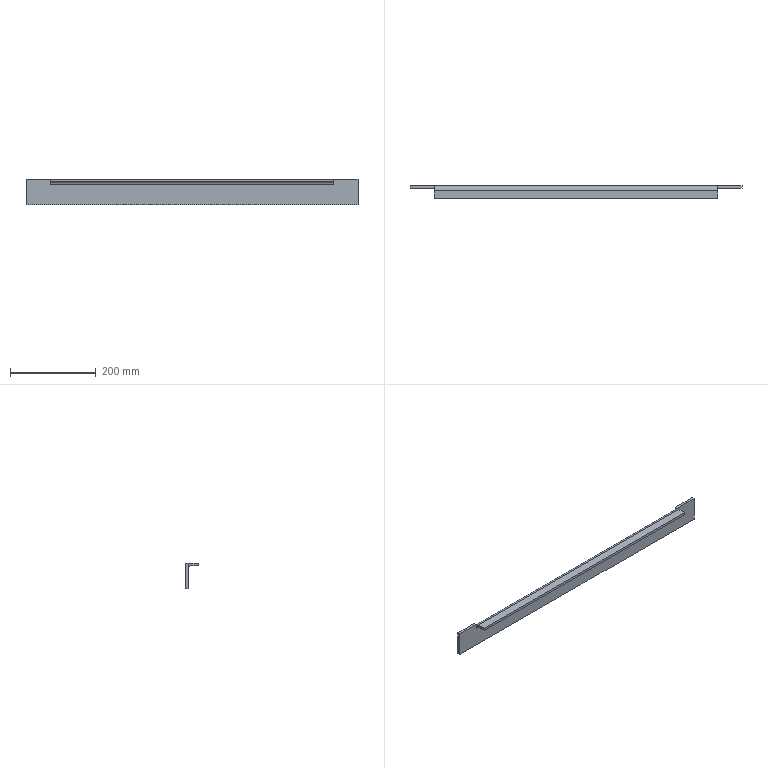Part | NX | features solid 2 | 1 solid | 18 faces | box 774 x 30 x 59 mm | volume 353589 mm3 | plane 16 | cylinder 2 | commonest cylinder face diameters 12 x1 24 x1
STEP:
#1=CARTESIAN_POINT('',(-1050.,491.,-219.));
#2=VERTEX_POINT('',#1);
#3=CARTESIAN_POINT('',(-390.,491.,-219.));
#4=VERTEX_POINT('',#3);
#5=CARTESIAN_POINT('',(-1050.,491.,-219.));
#6=DIRECTION('',(1.,0.,0.));
#7=VECTOR('',#6,1000.);
#8=LINE('',#5,#7);
#9=EDGE_CURVE('',#2,#4,#8,.T.);
#10=ORIENTED_EDGE('',*,*,#9,.T.);
#11=CARTESIAN_POINT('',(-390.,485.,-213.));
#12=VERTEX_POINT('',#11);
#13=CARTESIAN_POINT('',(-390.,485.,-219.));
#14=DIRECTION('',(-1.,0.,0.));
#15=DIRECTION('',(0.,1.,0.));
#16=AXIS2_PLACEMENT_3D('',#13,#14,#15);
#17=CIRCLE('',#16,6.);
#18=EDGE_CURVE('',#12,#4,#17,.T.);
#19=ORIENTED_EDGE('',*,*,#18,.F.);
#20=CARTESIAN_POINT('',(-1050.,485.,-213.));
#21=VERTEX_POINT('',#20);
#22=CARTESIAN_POINT('',(-390.,485.,-213.));
#23=DIRECTION('',(-1.,0.,0.));
#24=VECTOR('',#23,1000.);
#25=LINE('',#22,#24);
#26=EDGE_CURVE('',#12,#21,#25,.T.);
#27=ORIENTED_EDGE('',*,*,#26,.T.);
#28=CARTESIAN_POINT('',(-1050.,485.,-219.));
#29=DIRECTION('',(-1.,0.,0.));
#30=DIRECTION('',(0.,1.,0.));
#31=AXIS2_PLACEMENT_3D('',#28,#29,#30);
#32=CIRCLE('',#31,6.);
#33=EDGE_CURVE('',#21,#2,#32,.T.);
#34=ORIENTED_EDGE('',*,*,#33,.T.);
#35=EDGE_LOOP('',(#10,#19,#27,#34));
#36=FACE_BOUND('',#35,.T.);
#37=CARTESIAN_POINT('',(-1050.,485.,-219.));
#38=DIRECTION('',(1.,0.,0.));
#39=DIRECTION('',(0.,-1.,0.));
#40=AXIS2_PLACEMENT_3D('',#37,#38,#39);
#41=CYLINDRICAL_SURFACE('',#40,6.);
#42=ADVANCED_FACE('',(#36),#41,.F.);
#43=CARTESIAN_POINT('',(-1050.,497.,-219.));
#44=VERTEX_POINT('',#43);
#45=CARTESIAN_POINT('',(-390.,497.,-219.));
#46=VERTEX_POINT('',#45);
#47=CARTESIAN_POINT('',(-1050.,497.,-219.));
#48=DIRECTION('',(1.,0.,0.));
#49=VECTOR('',#48,1000.);
#50=LINE('',#47,#49);
#51=EDGE_CURVE('',#44,#46,#50,.T.);
#52=ORIENTED_EDGE('',*,*,#51,.F.);
#53=CARTESIAN_POINT('',(-1050.,485.,-207.));
#54=VERTEX_POINT('',#53);
#55=CARTESIAN_POINT('',(-1050.,485.,-219.));
#56=DIRECTION('',(-1.,0.,0.));
#57=DIRECTION('',(0.,-1.,0.));
#58=AXIS2_PLACEMENT_3D('',#55,#56,#57);
#59=CIRCLE('',#58,12.);
#60=EDGE_CURVE('',#54,#44,#59,.T.);
#61=ORIENTED_EDGE('',*,*,#60,.F.);
#62=CARTESIAN_POINT('',(-390.,485.,-207.));
#63=VERTEX_POINT('',#62);
#64=CARTESIAN_POINT('',(-390.,485.,-207.));
#65=DIRECTION('',(-1.,0.,0.));
#66=VECTOR('',#65,1000.);
#67=LINE('',#64,#66);
#68=EDGE_CURVE('',#63,#54,#67,.T.);
#69=ORIENTED_EDGE('',*,*,#68,.F.);
#70=CARTESIAN_POINT('',(-390.,485.,-219.));
#71=DIRECTION('',(-1.,0.,0.));
#72=DIRECTION('',(0.,-1.,0.));
#73=AXIS2_PLACEMENT_3D('',#70,#71,#72);
#74=CIRCLE('',#73,12.);
#75=EDGE_CURVE('',#63,#46,#74,.T.);
#76=ORIENTED_EDGE('',*,*,#75,.T.);
#77=EDGE_LOOP('',(#52,#61,#69,#76));
#78=FACE_BOUND('',#77,.T.);
#79=CARTESIAN_POINT('',(-1050.,485.,-219.));
#80=DIRECTION('',(1.,0.,0.));
#81=DIRECTION('',(0.,-1.,0.));
#82=AXIS2_PLACEMENT_3D('',#79,#80,#81);
#83=CYLINDRICAL_SURFACE('',#82,12.);
#84=ADVANCED_FACE('',(#78),#83,.T.);
#85=CARTESIAN_POINT('',(-1050.,467.,-213.));
#86=VERTEX_POINT('',#85);
#87=CARTESIAN_POINT('',(-390.,467.,-213.));
#88=VERTEX_POINT('',#87);
#89=CARTESIAN_POINT('',(-1050.,467.,-213.));
#90=DIRECTION('',(1.,0.,0.));
#91=VECTOR('',#90,1000.);
#92=LINE('',#89,#91);
#93=EDGE_CURVE('',#86,#88,#92,.T.);
#94=ORIENTED_EDGE('',*,*,#93,.T.);
#95=CARTESIAN_POINT('',(-390.,467.,-207.));
#96=VERTEX_POINT('',#95);
#97=CARTESIAN_POINT('',(-390.,467.,-207.));
#98=DIRECTION('',(0.,0.,-1.));
#99=VECTOR('',#98,1000.);
#100=LINE('',#97,#99);
#101=EDGE_CURVE('',#96,#88,#100,.T.);
#102=ORIENTED_EDGE('',*,*,#101,.F.);
#103=CARTESIAN_POINT('',(-1050.,467.,-207.));
#104=VERTEX_POINT('',#103);
#105=CARTESIAN_POINT('',(-1050.,467.,-207.));
#106=DIRECTION('',(1.,0.,0.));
#107=VECTOR('',#106,1000.);
#108=LINE('',#105,#107);
#109=EDGE_CURVE('',#104,#96,#108,.T.);
#110=ORIENTED_EDGE('',*,*,#109,.F.);
#111=CARTESIAN_POINT('',(-1050.,467.,-207.));
#112=DIRECTION('',(0.,0.,-1.));
#113=VECTOR('',#112,1000.);
#114=LINE('',#111,#113);
#115=EDGE_CURVE('',#104,#86,#114,.T.);
#116=ORIENTED_EDGE('',*,*,#115,.T.);
#117=EDGE_LOOP('',(#94,#102,#110,#116));
#118=FACE_BOUND('',#117,.T.);
#119=CARTESIAN_POINT('',(-1050.,467.,-207.));
#120=DIRECTION('',(0.,1.,0.));
#121=DIRECTION('',(1.,0.,0.));
#122=AXIS2_PLACEMENT_3D('',#119,#120,#121);
#123=PLANE('',#122);
#124=ADVANCED_FACE('',(#118),#123,.F.);
#125=ORIENTED_EDGE('',*,*,#26,.F.);
#126=CARTESIAN_POINT('',(-390.,492.069,-213.));
#127=DIRECTION('',(0.,1.,0.));
#128=VECTOR('',#127,1000.);
#129=LINE('',#126,#128);
#130=EDGE_CURVE('',#88,#12,#129,.T.);
#131=ORIENTED_EDGE('',*,*,#130,.F.);
#132=ORIENTED_EDGE('',*,*,#93,.F.);
#133=CARTESIAN_POINT('',(-1050.,492.069,-213.));
#134=DIRECTION('',(0.,-1.,0.));
#135=VECTOR('',#134,1000.);
#136=LINE('',#133,#135);
#137=EDGE_CURVE('',#21,#86,#136,.T.);
#138=ORIENTED_EDGE('',*,*,#137,.F.);
#139=EDGE_LOOP('',(#125,#131,#132,#138));
#140=FACE_BOUND('',#139,.T.);
#141=CARTESIAN_POINT('',(-1034.434,499.,-213.));
#142=DIRECTION('',(0.,0.,1.));
#143=DIRECTION('',(0.,-1.,0.));
#144=AXIS2_PLACEMENT_3D('',#141,#142,#143);
#145=PLANE('',#144);
#146=ADVANCED_FACE('',(#140),#145,.F.);
#147=CARTESIAN_POINT('',(-390.,492.069,-207.));
#148=DIRECTION('',(0.,1.,0.));
#149=VECTOR('',#148,1000.);
#150=LINE('',#147,#149);
#151=EDGE_CURVE('',#96,#63,#150,.T.);
#152=ORIENTED_EDGE('',*,*,#151,.T.);
#153=ORIENTED_EDGE('',*,*,#68,.T.);
#154=CARTESIAN_POINT('',(-1050.,492.069,-207.));
#155=DIRECTION('',(0.,-1.,0.));
#156=VECTOR('',#155,1000.);
#157=LINE('',#154,#156);
#158=EDGE_CURVE('',#54,#104,#157,.T.);
#159=ORIENTED_EDGE('',*,*,#158,.T.);
#160=ORIENTED_EDGE('',*,*,#109,.T.);
#161=EDGE_LOOP('',(#152,#153,#159,#160));
#162=FACE_BOUND('',#161,.T.);
#163=CARTESIAN_POINT('',(-1034.434,499.,-207.));
#164=DIRECTION('',(0.,0.,1.));
#165=DIRECTION('',(0.,-1.,0.));
#166=AXIS2_PLACEMENT_3D('',#163,#164,#165);
#167=PLANE('',#166);
#168=ADVANCED_FACE('',(#162),#167,.T.);
#169=CARTESIAN_POINT('',(-389.,491.,-219.5));
#170=VERTEX_POINT('',#169);
#171=CARTESIAN_POINT('',(-389.,497.,-219.5));
#172=VERTEX_POINT('',#171);
#173=CARTESIAN_POINT('',(-389.,497.,-219.5));
#174=DIRECTION('',(0.,1.,0.));
#175=VECTOR('',#174,1000.);
#176=LINE('',#173,#175);
#177=EDGE_CURVE('',#170,#172,#176,.T.);
#178=ORIENTED_EDGE('',*,*,#177,.T.);
#179=CARTESIAN_POINT('',(-390.,497.,-219.5));
#180=VERTEX_POINT('',#179);
#181=CARTESIAN_POINT('',(-389.,497.,-219.5));
#182=DIRECTION('',(1.,0.,0.));
#183=VECTOR('',#182,1000.);
#184=LINE('',#181,#183);
#185=EDGE_CURVE('',#180,#172,#184,.T.);
#186=ORIENTED_EDGE('',*,*,#185,.F.);
#187=CARTESIAN_POINT('',(-390.,491.,-219.5));
#188=VERTEX_POINT('',#187);
#189=CARTESIAN_POINT('',(-390.,497.,-219.5));
#190=DIRECTION('',(0.,1.,0.));
#191=VECTOR('',#190,1000.);
#192=LINE('',#189,#191);
#193=EDGE_CURVE('',#188,#180,#192,.T.);
#194=ORIENTED_EDGE('',*,*,#193,.F.);
#195=CARTESIAN_POINT('',(-390.,491.,-219.5));
#196=DIRECTION('',(1.,0.,0.));
#197=VECTOR('',#196,1000.);
#198=LINE('',#195,#197);
#199=EDGE_CURVE('',#188,#170,#198,.T.);
#200=ORIENTED_EDGE('',*,*,#199,.T.);
#201=EDGE_LOOP('',(#178,#186,#194,#200));
#202=FACE_BOUND('',#201,.T.);
#203=CARTESIAN_POINT('',(-389.,497.,-219.5));
#204=DIRECTION('',(0.,0.,-1.));
#205=DIRECTION('',(0.,-1.,0.));
#206=AXIS2_PLACEMENT_3D('',#203,#204,#205);
#207=PLANE('',#206);
#208=ADVANCED_FACE('',(#202),#207,.F.);
#209=CARTESIAN_POINT('',(-389.,491.,-207.));
#210=VERTEX_POINT('',#209);
#211=CARTESIAN_POINT('',(-389.,497.,-207.));
#212=VERTEX_POINT('',#211);
#213=CARTESIAN_POINT('',(-389.,497.,-207.));
#214=DIRECTION('',(0.,1.,0.));
#215=VECTOR('',#214,1000.);
#216=LINE('',#213,#215);
#217=EDGE_CURVE('',#210,#212,#216,.T.);
#218=ORIENTED_EDGE('',*,*,#217,.T.);
#219=CARTESIAN_POINT('',(-389.,497.,-207.));
#220=DIRECTION('',(0.,0.,1.));
#221=VECTOR('',#220,1000.);
#222=LINE('',#219,#221);
#223=EDGE_CURVE('',#172,#212,#222,.T.);
#224=ORIENTED_EDGE('',*,*,#223,.F.);
#225=ORIENTED_EDGE('',*,*,#177,.F.);
#226=CARTESIAN_POINT('',(-389.,491.,-219.5));
#227=DIRECTION('',(0.,0.,1.));
#228=VECTOR('',#227,1000.);
#229=LINE('',#226,#228);
#230=EDGE_CURVE('',#170,#210,#229,.T.);
#231=ORIENTED_EDGE('',*,*,#230,.T.);
#232=EDGE_LOOP('',(#218,#224,#225,#231));
#233=FACE_BOUND('',#232,.T.);
#234=CARTESIAN_POINT('',(-389.,497.,-207.));
#235=DIRECTION('',(1.,0.,0.));
#236=DIRECTION('',(0.,-1.,0.));
#237=AXIS2_PLACEMENT_3D('',#234,#235,#236);
#238=PLANE('',#237);
#239=ADVANCED_FACE('',(#233),#238,.F.);
#240=CARTESIAN_POINT('',(-1050.,491.,-219.5));
#241=VERTEX_POINT('',#240);
#242=CARTESIAN_POINT('',(-1051.,491.,-219.5));
#243=VERTEX_POINT('',#242);
#244=CARTESIAN_POINT('',(-1050.,491.,-219.5));
#245=DIRECTION('',(-1.,0.,0.));
#246=VECTOR('',#245,1000.);
#247=LINE('',#244,#246);
#248=EDGE_CURVE('',#241,#243,#247,.T.);
#249=ORIENTED_EDGE('',*,*,#248,.F.);
#250=CARTESIAN_POINT('',(-1050.,497.,-219.5));
#251=VERTEX_POINT('',#250);
#252=CARTESIAN_POINT('',(-1050.,497.,-219.5));
#253=DIRECTION('',(0.,1.,0.));
#254=VECTOR('',#253,1000.);
#255=LINE('',#252,#254);
#256=EDGE_CURVE('',#241,#251,#255,.T.);
#257=ORIENTED_EDGE('',*,*,#256,.T.);
#258=CARTESIAN_POINT('',(-1051.,497.,-219.5));
#259=VERTEX_POINT('',#258);
#260=CARTESIAN_POINT('',(-1051.,497.,-219.5));
#261=DIRECTION('',(-1.,0.,0.));
#262=VECTOR('',#261,1000.);
#263=LINE('',#260,#262);
#264=EDGE_CURVE('',#251,#259,#263,.T.);
#265=ORIENTED_EDGE('',*,*,#264,.T.);
#266=CARTESIAN_POINT('',(-1051.,497.,-219.5));
#267=DIRECTION('',(0.,1.,0.));
#268=VECTOR('',#267,1000.);
#269=LINE('',#266,#268);
#270=EDGE_CURVE('',#243,#259,#269,.T.);
#271=ORIENTED_EDGE('',*,*,#270,.F.);
#272=EDGE_LOOP('',(#249,#257,#265,#271));
#273=FACE_BOUND('',#272,.T.);
#274=CARTESIAN_POINT('',(-1051.,497.,-219.5));
#275=DIRECTION('',(0.,0.,-1.));
#276=DIRECTION('',(0.,-1.,0.));
#277=AXIS2_PLACEMENT_3D('',#274,#275,#276);
#278=PLANE('',#277);
#279=ADVANCED_FACE('',(#273),#278,.F.);
#280=ORIENTED_EDGE('',*,*,#270,.T.);
#281=CARTESIAN_POINT('',(-1051.,497.,-207.));
#282=VERTEX_POINT('',#281);
#283=CARTESIAN_POINT('',(-1051.,497.,-207.));
#284=DIRECTION('',(0.,0.,1.));
#285=VECTOR('',#284,1000.);
#286=LINE('',#283,#285);
#287=EDGE_CURVE('',#259,#282,#286,.T.);
#288=ORIENTED_EDGE('',*,*,#287,.T.);
#289=CARTESIAN_POINT('',(-1051.,491.,-207.));
#290=VERTEX_POINT('',#289);
#291=CARTESIAN_POINT('',(-1051.,497.,-207.));
#292=DIRECTION('',(0.,1.,0.));
#293=VECTOR('',#292,1000.);
#294=LINE('',#291,#293);
#295=EDGE_CURVE('',#290,#282,#294,.T.);
#296=ORIENTED_EDGE('',*,*,#295,.F.);
#297=CARTESIAN_POINT('',(-1051.,491.,-219.5));
#298=DIRECTION('',(0.,0.,1.));
#299=VECTOR('',#298,1000.);
#300=LINE('',#297,#299);
#301=EDGE_CURVE('',#243,#290,#300,.T.);
#302=ORIENTED_EDGE('',*,*,#301,.F.);
#303=EDGE_LOOP('',(#280,#288,#296,#302));
#304=FACE_BOUND('',#303,.T.);
#305=CARTESIAN_POINT('',(-1051.,497.,-207.));
#306=DIRECTION('',(-1.,0.,0.));
#307=DIRECTION('',(0.,0.,1.));
#308=AXIS2_PLACEMENT_3D('',#305,#306,#307);
#309=PLANE('',#308);
#310=ADVANCED_FACE('',(#304),#309,.F.);
#311=CARTESIAN_POINT('',(-333.,497.,-207.));
#312=VERTEX_POINT('',#311);
#313=CARTESIAN_POINT('',(-333.,491.,-207.));
#314=VERTEX_POINT('',#313);
#315=CARTESIAN_POINT('',(-333.,499.,-207.));
#316=DIRECTION('',(0.,-1.,0.));
#317=VECTOR('',#316,1000.);
#318=LINE('',#315,#317);
#319=EDGE_CURVE('',#312,#314,#318,.T.);
#320=ORIENTED_EDGE('',*,*,#319,.T.);
#321=CARTESIAN_POINT('',(-333.,491.,-266.));
#322=VERTEX_POINT('',#321);
#323=CARTESIAN_POINT('',(-333.,491.,-282.5));
#324=DIRECTION('',(0.,0.,1.));
#325=VECTOR('',#324,1000.);
#326=LINE('',#323,#325);
#327=EDGE_CURVE('',#322,#314,#326,.T.);
#328=ORIENTED_EDGE('',*,*,#327,.F.);
#329=CARTESIAN_POINT('',(-333.,497.,-266.));
#330=VERTEX_POINT('',#329);
#331=CARTESIAN_POINT('',(-333.,499.,-266.));
#332=DIRECTION('',(0.,1.,0.));
#333=VECTOR('',#332,1000.);
#334=LINE('',#331,#333);
#335=EDGE_CURVE('',#322,#330,#334,.T.);
#336=ORIENTED_EDGE('',*,*,#335,.T.);
#337=CARTESIAN_POINT('',(-333.,497.,-282.5));
#338=DIRECTION('',(0.,0.,1.));
#339=VECTOR('',#338,1000.);
#340=LINE('',#337,#339);
#341=EDGE_CURVE('',#330,#312,#340,.T.);
#342=ORIENTED_EDGE('',*,*,#341,.T.);
#343=EDGE_LOOP('',(#320,#328,#336,#342));
#344=FACE_BOUND('',#343,.T.);
#345=CARTESIAN_POINT('',(-333.,499.,-282.5));
#346=DIRECTION('',(-1.,0.,0.));
#347=DIRECTION('',(0.,0.,1.));
#348=AXIS2_PLACEMENT_3D('',#345,#346,#347);
#349=PLANE('',#348);
#350=ADVANCED_FACE('',(#344),#349,.F.);
#351=ORIENTED_EDGE('',*,*,#9,.F.);
#352=CARTESIAN_POINT('',(-1050.,491.,-219.5));
#353=DIRECTION('',(0.,0.,-1.));
#354=VECTOR('',#353,1000.);
#355=LINE('',#352,#354);
#356=EDGE_CURVE('',#2,#241,#355,.T.);
#357=ORIENTED_EDGE('',*,*,#356,.T.);
#358=ORIENTED_EDGE('',*,*,#248,.T.);
#359=ORIENTED_EDGE('',*,*,#301,.T.);
#360=CARTESIAN_POINT('',(-1107.,491.,-207.));
#361=VERTEX_POINT('',#360);
#362=CARTESIAN_POINT('',(-1090.,491.,-207.));
#363=DIRECTION('',(-1.,0.,0.));
#364=VECTOR('',#363,1000.);
#365=LINE('',#362,#364);
#366=EDGE_CURVE('',#290,#361,#365,.T.);
#367=ORIENTED_EDGE('',*,*,#366,.T.);
#368=CARTESIAN_POINT('',(-1107.,491.,-266.));
#369=VERTEX_POINT('',#368);
#370=CARTESIAN_POINT('',(-1107.,491.,-282.5));
#371=DIRECTION('',(0.,0.,-1.));
#372=VECTOR('',#371,1000.);
#373=LINE('',#370,#372);
#374=EDGE_CURVE('',#361,#369,#373,.T.);
#375=ORIENTED_EDGE('',*,*,#374,.T.);
#376=CARTESIAN_POINT('',(-1090.,491.,-266.));
#377=DIRECTION('',(1.,0.,0.));
#378=VECTOR('',#377,1000.);
#379=LINE('',#376,#378);
#380=EDGE_CURVE('',#369,#322,#379,.T.);
#381=ORIENTED_EDGE('',*,*,#380,.T.);
#382=ORIENTED_EDGE('',*,*,#327,.T.);
#383=CARTESIAN_POINT('',(-1090.,491.,-207.));
#384=DIRECTION('',(-1.,0.,0.));
#385=VECTOR('',#384,1000.);
#386=LINE('',#383,#385);
#387=EDGE_CURVE('',#314,#210,#386,.T.);
#388=ORIENTED_EDGE('',*,*,#387,.T.);
#389=ORIENTED_EDGE('',*,*,#230,.F.);
#390=ORIENTED_EDGE('',*,*,#199,.F.);
#391=CARTESIAN_POINT('',(-390.,491.,-219.5));
#392=DIRECTION('',(0.,0.,-1.));
#393=VECTOR('',#392,1000.);
#394=LINE('',#391,#393);
#395=EDGE_CURVE('',#4,#188,#394,.T.);
#396=ORIENTED_EDGE('',*,*,#395,.F.);
#397=EDGE_LOOP('',(#351,#357,#358,#359,#367,#375,#381,#382,#388,#389,#390,#396));
#398=FACE_BOUND('',#397,.T.);
#399=CARTESIAN_POINT('',(-1090.,491.,-282.5));
#400=DIRECTION('',(0.,-1.,0.));
#401=DIRECTION('',(-1.,0.,0.));
#402=AXIS2_PLACEMENT_3D('',#399,#400,#401);
#403=PLANE('',#402);
#404=ADVANCED_FACE('',(#398),#403,.T.);
#405=ORIENTED_EDGE('',*,*,#335,.F.);
#406=ORIENTED_EDGE('',*,*,#380,.F.);
#407=CARTESIAN_POINT('',(-1107.,497.,-266.));
#408=VERTEX_POINT('',#407);
#409=CARTESIAN_POINT('',(-1107.,499.,-266.));
#410=DIRECTION('',(0.,1.,0.));
#411=VECTOR('',#410,1000.);
#412=LINE('',#409,#411);
#413=EDGE_CURVE('',#369,#408,#412,.T.);
#414=ORIENTED_EDGE('',*,*,#413,.T.);
#415=CARTESIAN_POINT('',(-1090.,497.,-266.));
#416=DIRECTION('',(1.,0.,0.));
#417=VECTOR('',#416,1000.);
#418=LINE('',#415,#417);
#419=EDGE_CURVE('',#408,#330,#418,.T.);
#420=ORIENTED_EDGE('',*,*,#419,.T.);
#421=EDGE_LOOP('',(#405,#406,#414,#420));
#422=FACE_BOUND('',#421,.T.);
#423=CARTESIAN_POINT('',(-1090.,499.,-266.));
#424=DIRECTION('',(0.,0.,1.));
#425=DIRECTION('',(0.,-1.,0.));
#426=AXIS2_PLACEMENT_3D('',#423,#424,#425);
#427=PLANE('',#426);
#428=ADVANCED_FACE('',(#422),#427,.F.);
#429=ORIENTED_EDGE('',*,*,#413,.F.);
#430=ORIENTED_EDGE('',*,*,#374,.F.);
#431=CARTESIAN_POINT('',(-1107.,497.,-207.));
#432=VERTEX_POINT('',#431);
#433=CARTESIAN_POINT('',(-1107.,491.,-207.));
#434=DIRECTION('',(0.,-1.,0.));
#435=VECTOR('',#434,1000.);
#436=LINE('',#433,#435);
#437=EDGE_CURVE('',#432,#361,#436,.T.);
#438=ORIENTED_EDGE('',*,*,#437,.F.);
#439=CARTESIAN_POINT('',(-1107.,497.,-282.5));
#440=DIRECTION('',(0.,0.,1.));
#441=VECTOR('',#440,1000.);
#442=LINE('',#439,#441);
#443=EDGE_CURVE('',#408,#432,#442,.T.);
#444=ORIENTED_EDGE('',*,*,#443,.F.);
#445=EDGE_LOOP('',(#429,#430,#438,#444));
#446=FACE_BOUND('',#445,.T.);
#447=CARTESIAN_POINT('',(-1107.,499.,-282.5));
#448=DIRECTION('',(1.,0.,0.));
#449=DIRECTION('',(0.,-1.,0.));
#450=AXIS2_PLACEMENT_3D('',#447,#448,#449);
#451=PLANE('',#450);
#452=ADVANCED_FACE('',(#446),#451,.F.);
#453=ORIENTED_EDGE('',*,*,#366,.F.);
#454=ORIENTED_EDGE('',*,*,#295,.T.);
#455=CARTESIAN_POINT('',(-1090.,497.,-207.));
#456=DIRECTION('',(-1.,0.,0.));
#457=VECTOR('',#456,1000.);
#458=LINE('',#455,#457);
#459=EDGE_CURVE('',#282,#432,#458,.T.);
#460=ORIENTED_EDGE('',*,*,#459,.T.);
#461=ORIENTED_EDGE('',*,*,#437,.T.);
#462=EDGE_LOOP('',(#453,#454,#460,#461));
#463=FACE_BOUND('',#462,.T.);
#464=CARTESIAN_POINT('',(-1090.,491.,-207.));
#465=DIRECTION('',(0.,0.,-1.));
#466=DIRECTION('',(0.,-1.,0.));
#467=AXIS2_PLACEMENT_3D('',#464,#465,#466);
#468=PLANE('',#467);
#469=ADVANCED_FACE('',(#463),#468,.F.);
#470=CARTESIAN_POINT('',(-1090.,497.,-207.));
#471=DIRECTION('',(-1.,0.,0.));
#472=VECTOR('',#471,1000.);
#473=LINE('',#470,#472);
#474=EDGE_CURVE('',#312,#212,#473,.T.);
#475=ORIENTED_EDGE('',*,*,#474,.T.);
#476=ORIENTED_EDGE('',*,*,#217,.F.);
#477=ORIENTED_EDGE('',*,*,#387,.F.);
#478=ORIENTED_EDGE('',*,*,#319,.F.);
#479=EDGE_LOOP('',(#475,#476,#477,#478));
#480=FACE_BOUND('',#479,.T.);
#481=CARTESIAN_POINT('',(-1090.,491.,-207.));
#482=DIRECTION('',(0.,0.,-1.));
#483=DIRECTION('',(0.,-1.,0.));
#484=AXIS2_PLACEMENT_3D('',#481,#482,#483);
#485=PLANE('',#484);
#486=ADVANCED_FACE('',(#480),#485,.F.);
#487=CARTESIAN_POINT('',(-1050.,497.,-207.));
#488=DIRECTION('',(0.,0.,-1.));
#489=VECTOR('',#488,1000.);
#490=LINE('',#487,#489);
#491=EDGE_CURVE('',#44,#251,#490,.T.);
#492=ORIENTED_EDGE('',*,*,#491,.F.);
#493=ORIENTED_EDGE('',*,*,#51,.T.);
#494=CARTESIAN_POINT('',(-390.,497.,-207.));
#495=DIRECTION('',(0.,0.,-1.));
#496=VECTOR('',#495,1000.);
#497=LINE('',#494,#496);
#498=EDGE_CURVE('',#46,#180,#497,.T.);
#499=ORIENTED_EDGE('',*,*,#498,.T.);
#500=ORIENTED_EDGE('',*,*,#185,.T.);
#501=ORIENTED_EDGE('',*,*,#223,.T.);
#502=ORIENTED_EDGE('',*,*,#474,.F.);
#503=ORIENTED_EDGE('',*,*,#341,.F.);
#504=ORIENTED_EDGE('',*,*,#419,.F.);
#505=ORIENTED_EDGE('',*,*,#443,.T.);
#506=ORIENTED_EDGE('',*,*,#459,.F.);
#507=ORIENTED_EDGE('',*,*,#287,.F.);
#508=ORIENTED_EDGE('',*,*,#264,.F.);
#509=EDGE_LOOP('',(#492,#493,#499,#500,#501,#502,#503,#504,#505,#506,#507,#508));
#510=FACE_BOUND('',#509,.T.);
#511=CARTESIAN_POINT('',(-1090.,497.,-282.5));
#512=DIRECTION('',(0.,-1.,0.));
#513=DIRECTION('',(-1.,0.,0.));
#514=AXIS2_PLACEMENT_3D('',#511,#512,#513);
#515=PLANE('',#514);
#516=ADVANCED_FACE('',(#510),#515,.F.);
#517=ORIENTED_EDGE('',*,*,#498,.F.);
#518=ORIENTED_EDGE('',*,*,#75,.F.);
#519=ORIENTED_EDGE('',*,*,#151,.F.);
#520=ORIENTED_EDGE('',*,*,#101,.T.);
#521=ORIENTED_EDGE('',*,*,#130,.T.);
#522=ORIENTED_EDGE('',*,*,#18,.T.);
#523=ORIENTED_EDGE('',*,*,#395,.T.);
#524=ORIENTED_EDGE('',*,*,#193,.T.);
#525=EDGE_LOOP('',(#517,#518,#519,#520,#521,#522,#523,#524));
#526=FACE_BOUND('',#525,.T.);
#527=CARTESIAN_POINT('',(-390.,497.,-207.));
#528=DIRECTION('',(-1.,0.,0.));
#529=DIRECTION('',(0.,0.,1.));
#530=AXIS2_PLACEMENT_3D('',#527,#528,#529);
#531=PLANE('',#530);
#532=ADVANCED_FACE('',(#526),#531,.F.);
#533=ORIENTED_EDGE('',*,*,#356,.F.);
#534=ORIENTED_EDGE('',*,*,#33,.F.);
#535=ORIENTED_EDGE('',*,*,#137,.T.);
#536=ORIENTED_EDGE('',*,*,#115,.F.);
#537=ORIENTED_EDGE('',*,*,#158,.F.);
#538=ORIENTED_EDGE('',*,*,#60,.T.);
#539=ORIENTED_EDGE('',*,*,#491,.T.);
#540=ORIENTED_EDGE('',*,*,#256,.F.);
#541=EDGE_LOOP('',(#533,#534,#535,#536,#537,#538,#539,#540));
#542=FACE_BOUND('',#541,.T.);
#543=CARTESIAN_POINT('',(-1050.,497.,-207.));
#544=DIRECTION('',(1.,0.,0.));
#545=DIRECTION('',(0.,-1.,0.));
#546=AXIS2_PLACEMENT_3D('',#543,#544,#545);
#547=PLANE('',#546);
#548=ADVANCED_FACE('',(#542),#547,.F.);
#549=CLOSED_SHELL('',(#42,#84,#124,#146,#168,#208,#239,#279,#310,#350,#404,#428,#452,#469,#486,#516,#532,#548));
#550=MANIFOLD_SOLID_BREP('',#549);
#551=(LENGTH_UNIT()NAMED_UNIT(*)SI_UNIT(.MILLI.,.METRE.));
#552=UNCERTAINTY_MEASURE_WITH_UNIT(LENGTH_MEASURE(0.00001),#551,'','');
#553=(NAMED_UNIT(*)PLANE_ANGLE_UNIT()SI_UNIT($,.RADIAN.));
#554=(NAMED_UNIT(*)SI_UNIT($,.STERADIAN.)SOLID_ANGLE_UNIT());
#555=(GEOMETRIC_REPRESENTATION_CONTEXT(3)GLOBAL_UNCERTAINTY_ASSIGNED_CONTEXT((#552))GLOBAL_UNIT_ASSIGNED_CONTEXT((#551,#553,#554))REPRESENTATION_CONTEXT('',''));
#556=ADVANCED_BREP_SHAPE_REPRESENTATION('',(#550),#555);